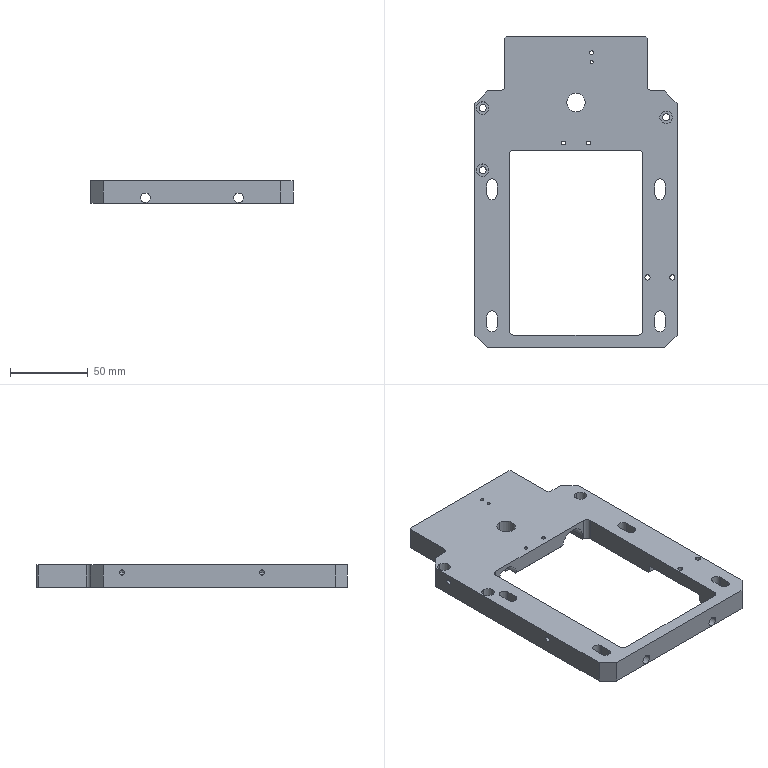NC program | NX | posted with a generic post | part box 130 x 200 x 14.5 mm
Whole program:
N10 G17 G21 G94 G90
(DRILLING_COPY_2 , TOOL : ZXZ)
N12 T21 M6
N14 G54
N16 G17 G0 G90 X15. Y-0.75 B0. C0. S3500 M3
N18 G43 Z30. H21
N20 G94 G81 G98 Z-1. F250. R3.
N22 X-15.
N24 X42.5
N26 X-42.5
N28 G80
N30 G0 X-42.5 Y-0.75 Z30.
N32 M5
(DRILLING_COPY_1_COPY_1 , TOOL : 3.3ZT)
N34 T13 M6
N36 G54
N38 G17 G0 G90 X15. Y-0.75 B0. C0. S2000 M3
N40 G43 Z30. H13
N42 G94 G83 G98 Z-15.091 F150. Q2. R3.
N44 X-15.
N46 G80
N48 G0 X-15. Y-0.75 Z30.
N50 M5
(DRILLING_COPY_COPY_COPY , TOOL : 2.5ZT)
N52 T22 M6
N54 G54
N56 G17 G0 G90 X-42.5 Y-0.75 B0. C0. S2000 M3
N58 G43 Z30. H22
N60 G94 G83 G98 Z-5. F150. Q2. R3.
N62 X42.5
N64 G80
N66 G0 X42.5 Y-0.75 Z30.
N68 M5
(HOLE_MILLING_2 , TOOL : D2)
N70 T18 M6
N72 G54
N74 G17 G0 G90 X-42.5 Y-0.75 B0. C0. S7500 M3
N76 G43 Z30. H18
N78 Z0.5
N80 G94 G3 X-42.735 Y-0.515 R0.235 F800.
N82 X-42.97 Y-0.75 R0.235
N84 X-42.97 Y-0.75 Z0.475 I0.47 J0.
N86 X-42.97 Y-0.75 Z0.45 I0.47 J0.
N88 X-42.97 Y-0.75 Z0.425 I0.47 J0.
N90 X-42.97 Y-0.75 Z0.4 I0.47 J0.
N92 X-42.97 Y-0.75 Z0.375 I0.47 J0.
N94 X-42.97 Y-0.75 Z0.35 I0.47 J0.
N96 X-42.97 Y-0.75 Z0.325 I0.47 J0.
N98 X-42.97 Y-0.75 Z0.3 I0.47 J0.
N100 X-42.97 Y-0.75 Z0.275 I0.47 J0.
N102 X-42.97 Y-0.75 Z0.25 I0.47 J0.
N104 X-42.97 Y-0.75 Z0.225 I0.47 J0.
N106 X-42.97 Y-0.75 Z0.2 I0.47 J0.
N108 X-42.97 Y-0.75 Z0.175 I0.47 J0.
N110 X-42.97 Y-0.75 Z0.15 I0.47 J0.
N112 X-42.97 Y-0.75 Z0.125 I0.47 J0.
N114 X-42.97 Y-0.75 Z0.1 I0.47 J0.
N116 X-42.97 Y-0.75 Z0.075 I0.47 J0.
N118 X-42.97 Y-0.75 Z0.05 I0.47 J0.
N120 X-42.97 Y-0.75 Z0.025 I0.47 J0.
N122 X-42.97 Y-0.75 Z0. I0.47 J0.
N124 X-42.97 Y-0.75 Z-0.025 I0.47 J0.
N126 X-42.97 Y-0.75 Z-0.05 I0.47 J0.
N128 X-42.97 Y-0.75 Z-0.075 I0.47 J0.
N130 X-42.97 Y-0.75 Z-0.1 I0.47 J0.
N132 X-42.97 Y-0.75 Z-0.125 I0.47 J0.
N134 X-42.97 Y-0.75 Z-0.15 I0.47 J0.
N136 X-42.97 Y-0.75 Z-0.175 I0.47 J0.
N138 X-42.97 Y-0.75 Z-0.2 I0.47 J0.
N140 X-42.97 Y-0.75 Z-0.225 I0.47 J0.
N142 X-42.97 Y-0.75 Z-0.25 I0.47 J0.
N144 X-42.97 Y-0.75 Z-0.275 I0.47 J0.
N146 X-42.97 Y-0.75 Z-0.3 I0.47 J0.
N148 X-42.97 Y-0.75 Z-0.325 I0.47 J0.
N150 X-42.97 Y-0.75 Z-0.35 I0.47 J0.
N152 X-42.97 Y-0.75 Z-0.375 I0.47 J0.
N154 X-42.97 Y-0.75 Z-0.4 I0.47 J0.
N156 X-42.97 Y-0.75 Z-0.425 I0.47 J0.
N158 X-42.97 Y-0.75 Z-0.45 I0.47 J0.
N160 X-42.97 Y-0.75 Z-0.475 I0.47 J0.
N162 X-42.97 Y-0.75 Z-0.5 I0.47 J0.
N164 X-42.97 Y-0.75 Z-0.525 I0.47 J0.
N166 X-42.97 Y-0.75 Z-0.55 I0.47 J0.
N168 X-42.97 Y-0.75 Z-0.575 I0.47 J0.
N170 X-42.97 Y-0.75 Z-0.6 I0.47 J0.
N172 X-42.97 Y-0.75 Z-0.625 I0.47 J0.
N174 X-42.97 Y-0.75 Z-0.65 I0.47 J0.
N176 X-42.97 Y-0.75 Z-0.675 I0.47 J0.
N178 X-42.97 Y-0.75 Z-0.7 I0.47 J0.
N180 X-42.97 Y-0.75 Z-0.725 I0.47 J0.
N182 X-42.97 Y-0.75 Z-0.75 I0.47 J0.
N184 X-42.97 Y-0.75 Z-0.775 I0.47 J0.
N186 X-42.97 Y-0.75 Z-0.8 I0.47 J0.
N188 X-42.97 Y-0.75 Z-0.825 I0.47 J0.
N190 X-42.97 Y-0.75 Z-0.85 I0.47 J0.
N192 X-42.97 Y-0.75 Z-0.875 I0.47 J0.
N194 X-42.97 Y-0.75 Z-0.9 I0.47 J0.
N196 X-42.97 Y-0.75 Z-0.925 I0.47 J0.
N198 X-42.97 Y-0.75 Z-0.95 I0.47 J0.
N200 X-42.97 Y-0.75 Z-0.975 I0.47 J0.
N202 X-42.97 Y-0.75 Z-1. I0.47 J0.
N204 X-42.97 Y-0.75 Z-1.025 I0.47 J0.
N206 X-42.97 Y-0.75 Z-1.05 I0.47 J0.
N208 X-42.97 Y-0.75 Z-1.075 I0.47 J0.
N210 X-42.97 Y-0.75 Z-1.1 I0.47 J0.
N212 X-42.97 Y-0.75 Z-1.125 I0.47 J0.
N214 X-42.97 Y-0.75 Z-1.15 I0.47 J0.
N216 X-42.97 Y-0.75 Z-1.175 I0.47 J0.
N218 X-42.97 Y-0.75 Z-1.2 I0.47 J0.
N220 X-42.97 Y-0.75 Z-1.225 I0.47 J0.
N222 X-42.97 Y-0.75 Z-1.25 I0.47 J0.
N224 X-42.97 Y-0.75 Z-1.275 I0.47 J0.
N226 X-42.97 Y-0.75 Z-1.3 I0.47 J0.
N228 X-42.97 Y-0.75 Z-1.325 I0.47 J0.
N230 X-42.97 Y-0.75 Z-1.35 I0.47 J0.
N232 X-42.97 Y-0.75 Z-1.375 I0.47 J0.
N234 X-42.97 Y-0.75 Z-1.4 I0.47 J0.
N236 X-42.97 Y-0.75 Z-1.425 I0.47 J0.
N238 X-42.97 Y-0.75 Z-1.45 I0.47 J0.
N240 X-42.97 Y-0.75 Z-1.475 I0.47 J0.
N242 X-42.97 Y-0.75 Z-1.5 I0.47 J0.
N244 X-42.97 Y-0.75 Z-1.525 I0.47 J0.
N246 X-42.97 Y-0.75 Z-1.55 I0.47 J0.
N248 X-42.97 Y-0.75 Z-1.575 I0.47 J0.
N250 X-42.97 Y-0.75 Z-1.6 I0.47 J0.
N252 X-42.97 Y-0.75 Z-1.625 I0.47 J0.
N254 X-42.97 Y-0.75 Z-1.65 I0.47 J0.
N256 X-42.97 Y-0.75 Z-1.675 I0.47 J0.
N258 X-42.97 Y-0.75 Z-1.7 I0.47 J0.
N260 X-42.97 Y-0.75 Z-1.725 I0.47 J0.
N262 X-42.97 Y-0.75 Z-1.75 I0.47 J0.
N264 X-42.97 Y-0.75 Z-1.775 I0.47 J0.
N266 X-42.97 Y-0.75 Z-1.8 I0.47 J0.
N268 X-42.97 Y-0.75 Z-1.825 I0.47 J0.
N270 X-42.97 Y-0.75 Z-1.85 I0.47 J0.
N272 X-42.97 Y-0.75 Z-1.875 I0.47 J0.
N274 X-42.97 Y-0.75 Z-1.9 I0.47 J0.
N276 X-42.97 Y-0.75 Z-1.925 I0.47 J0.
N278 X-42.97 Y-0.75 Z-1.95 I0.47 J0.
N280 X-42.97 Y-0.75 Z-1.975 I0.47 J0.
N282 X-42.97 Y-0.75 Z-2. I0.47 J0.
N284 X-42.97 Y-0.75 Z-2.025 I0.47 J0.
N286 X-42.97 Y-0.75 Z-2.05 I0.47 J0.
N288 X-42.97 Y-0.75 Z-2.075 I0.47 J0.
N290 X-42.97 Y-0.75 Z-2.1 I0.47 J0.
N292 X-42.97 Y-0.75 Z-2.125 I0.47 J0.
N294 X-42.97 Y-0.75 Z-2.15 I0.47 J0.
N296 X-42.97 Y-0.75 Z-2.175 I0.47 J0.
N298 X-42.97 Y-0.75 Z-2.2 I0.47 J0.
N300 X-42.97 Y-0.75 Z-2.225 I0.47 J0.
N302 X-42.97 Y-0.75 Z-2.25 I0.47 J0.
N304 X-42.97 Y-0.75 Z-2.275 I0.47 J0.
N306 X-42.97 Y-0.75 Z-2.3 I0.47 J0.
N308 X-42.97 Y-0.75 Z-2.325 I0.47 J0.
N310 X-42.97 Y-0.75 Z-2.35 I0.47 J0.
N312 X-42.97 Y-0.75 Z-2.375 I0.47 J0.
N314 X-42.97 Y-0.75 Z-2.4 I0.47 J0.
N316 X-42.97 Y-0.75 Z-2.425 I0.47 J0.
N318 X-42.97 Y-0.75 Z-2.45 I0.47 J0.
N320 X-42.97 Y-0.75 Z-2.475 I0.47 J0.
N322 X-42.97 Y-0.75 Z-2.5 I0.47 J0.
N324 X-42.97 Y-0.75 Z-2.525 I0.47 J0.
N326 X-42.97 Y-0.75 Z-2.55 I0.47 J0.
N328 X-42.97 Y-0.75 Z-2.575 I0.47 J0.
N330 X-42.97 Y-0.75 Z-2.6 I0.47 J0.
N332 X-42.97 Y-0.75 Z-2.625 I0.47 J0.
N334 X-42.97 Y-0.75 Z-2.65 I0.47 J0.
N336 X-42.97 Y-0.75 Z-2.675 I0.47 J0.
N338 X-42.97 Y-0.75 Z-2.7 I0.47 J0.
N340 X-42.97 Y-0.75 Z-2.725 I0.47 J0.
N342 X-42.97 Y-0.75 Z-2.75 I0.47 J0.
N344 X-42.97 Y-0.75 Z-2.775 I0.47 J0.
N346 X-42.97 Y-0.75 Z-2.8 I0.47 J0.
N348 X-42.97 Y-0.75 Z-2.825 I0.47 J0.
N350 X-42.97 Y-0.75 Z-2.85 I0.47 J0.
N352 X-42.97 Y-0.75 Z-2.875 I0.47 J0.
N354 X-42.97 Y-0.75 Z-2.9 I0.47 J0.
N356 X-42.97 Y-0.75 Z-2.925 I0.47 J0.
N358 X-42.97 Y-0.75 Z-2.95 I0.47 J0.
N360 X-42.97 Y-0.75 Z-2.975 I0.47 J0.
N362 X-42.97 Y-0.75 Z-3. I0.47 J0.
N364 X-42.97 Y-0.75 Z-3.025 I0.47 J0.
N366 X-42.97 Y-0.75 Z-3.05 I0.47 J0.
N368 X-42.97 Y-0.75 Z-3.075 I0.47 J0.
N370 X-42.97 Y-0.75 Z-3.1 I0.47 J0.
N372 X-42.97 Y-0.75 Z-3.125 I0.47 J0.
N374 X-42.97 Y-0.75 Z-3.15 I0.47 J0.
N376 X-42.97 Y-0.75 Z-3.175 I0.47 J0.
N378 X-42.97 Y-0.75 Z-3.2 I0.47 J0.
N380 X-42.97 Y-0.75 Z-3.225 I0.47 J0.
N382 X-42.97 Y-0.75 Z-3.25 I0.47 J0.
N384 X-42.97 Y-0.75 Z-3.275 I0.47 J0.
N386 X-42.97 Y-0.75 Z-3.3 I0.47 J0.
N388 X-42.97 Y-0.75 Z-3.325 I0.47 J0.
N390 X-42.97 Y-0.75 Z-3.35 I0.47 J0.
N392 X-42.97 Y-0.75 Z-3.375 I0.47 J0.
N394 X-42.97 Y-0.75 Z-3.4 I0.47 J0.
N396 X-42.97 Y-0.75 Z-3.425 I0.47 J0.
N398 X-42.97 Y-0.75 Z-3.45 I0.47 J0.
N400 X-42.97 Y-0.75 Z-3.475 I0.47 J0.
N402 X-42.97 Y-0.75 Z-3.5 I0.47 J0.
N404 X-42.97 Y-0.75 Z-3.525 I0.47 J0.
N406 X-42.97 Y-0.75 Z-3.55 I0.47 J0.
N408 X-42.97 Y-0.75 Z-3.575 I0.47 J0.
N410 X-42.97 Y-0.75 Z-3.6 I0.47 J0.
N412 X-42.97 Y-0.75 Z-3.625 I0.47 J0.
N414 X-42.97 Y-0.75 Z-3.65 I0.47 J0.
N416 X-42.97 Y-0.75 Z-3.675 I0.47 J0.
N418 X-42.97 Y-0.75 Z-3.7 I0.47 J0.
N420 X-42.97 Y-0.75 Z-3.725 I0.47 J0.
N422 X-42.97 Y-0.75 Z-3.75 I0.47 J0.
N424 X-42.97 Y-0.75 Z-3.775 I0.47 J0.
N426 X-42.97 Y-0.75 Z-3.8 I0.47 J0.
N428 X-42.97 Y-0.75 Z-3.825 I0.47 J0.
N430 X-42.97 Y-0.75 Z-3.85 I0.47 J0.
N432 X-42.97 Y-0.75 Z-3.875 I0.47 J0.
N434 X-42.97 Y-0.75 Z-3.9 I0.47 J0.
N436 X-42.97 Y-0.75 Z-3.925 I0.47 J0.
N438 X-42.97 Y-0.75 Z-3.95 I0.47 J0.
N440 X-42.97 Y-0.75 Z-3.975 I0.47 J0.
N442 X-42.97 Y-0.75 Z-4. I0.47 J0.
N444 X-42.97 Y-0.75 Z-4.025 I0.47 J0.
N446 X-42.97 Y-0.75 Z-4.05 I0.47 J0.
N448 X-42.97 Y-0.75 Z-4.075 I0.47 J0.
N450 X-42.97 Y-0.75 Z-4.1 I0.47 J0.
N452 X-42.97 Y-0.75 Z-4.125 I0.47 J0.
N454 X-42.97 Y-0.75 Z-4.15 I0.47 J0.
N456 X-42.97 Y-0.75 Z-4.175 I0.47 J0.
N458 X-42.97 Y-0.75 Z-4.2 I0.47 J0.
N460 X-42.97 Y-0.75 Z-4.225 I0.47 J0.
N462 X-42.97 Y-0.75 Z-4.25 I0.47 J0.
N464 X-42.97 Y-0.75 Z-4.275 I0.47 J0.
N466 X-42.97 Y-0.75 Z-4.3 I0.47 J0.
N468 X-42.97 Y-0.75 Z-4.325 I0.47 J0.
N470 X-42.97 Y-0.75 Z-4.35 I0.47 J0.
N472 X-42.97 Y-0.75 Z-4.375 I0.47 J0.
N474 X-42.97 Y-0.75 Z-4.4 I0.47 J0.
N476 X-42.97 Y-0.75 Z-4.425 I0.47 J0.
N478 X-42.97 Y-0.75 Z-4.45 I0.47 J0.
N480 X-42.97 Y-0.75 Z-4.475 I0.47 J0.
N482 X-42.97 Y-0.75 Z-4.5 I0.47 J0.
N484 X-42.97 Y-0.75 Z-4.525 I0.47 J0.
N486 X-42.97 Y-0.75 Z-4.55 I0.47 J0.
N488 X-42.97 Y-0.75 Z-4.575 I0.47 J0.
N490 X-42.97 Y-0.75 Z-4.6 I0.47 J0.
N492 X-42.97 Y-0.75 Z-4.625 I0.47 J0.
N494 X-42.97 Y-0.75 Z-4.65 I0.47 J0.
N496 X-42.97 Y-0.75 Z-4.675 I0.47 J0.
N498 X-42.97 Y-0.75 Z-4.7 I0.47 J0.
N500 X-42.97 Y-0.75 Z-4.725 I0.47 J0.
N502 X-42.97 Y-0.75 Z-4.75 I0.47 J0.
N504 X-42.97 Y-0.75 Z-4.775 I0.47 J0.
N506 X-42.97 Y-0.75 Z-4.8 I0.47 J0.
N508 X-42.97 Y-0.75 Z-4.825 I0.47 J0.
N510 X-42.97 Y-0.75 Z-4.85 I0.47 J0.
N512 X-42.97 Y-0.75 Z-4.875 I0.47 J0.
N514 X-42.97 Y-0.75 Z-4.9 I0.47 J0.
N516 X-42.97 Y-0.75 Z-4.925 I0.47 J0.
N518 X-42.97 Y-0.75 Z-4.95 I0.47 J0.
N520 X-42.97 Y-0.75 Z-4.975 I0.47 J0.
N522 X-42.97 Y-0.75 Z-5. I0.47 J0.
N524 X-42.5 Y-1.22 R0.47
N526 X-42.97 Y-0.75 R-0.47
N528 X-42.735 Y-0.985 R0.235
N530 X-42.5 Y-0.75 R0.235
N532 G0 Z30.
N534 X42.5
N536 Z0.5
N538 G3 X42.265 Y-0.515 R0.235
N540 X42.03 Y-0.75 R0.235
N542 X42.03 Y-0.75 Z0.475 I0.47 J0.
N544 X42.03 Y-0.75 Z0.45 I0.47 J0.
N546 X42.03 Y-0.75 Z0.425 I0.47 J0.
N548 X42.03 Y-0.75 Z0.4 I0.47 J0.
N550 X42.03 Y-0.75 Z0.375 I0.47 J0.
N552 X42.03 Y-0.75 Z0.35 I0.47 J0.
N554 X42.03 Y-0.75 Z0.325 I0.47 J0.
N556 X42.03 Y-0.75 Z0.3 I0.47 J0.
N558 X42.03 Y-0.75 Z0.275 I0.47 J0.
N560 X42.03 Y-0.75 Z0.25 I0.47 J0.
N562 X42.03 Y-0.75 Z0.225 I0.47 J0.
N564 X42.03 Y-0.75 Z0.2 I0.47 J0.
N566 X42.03 Y-0.75 Z0.175 I0.47 J0.
N568 X42.03 Y-0.75 Z0.15 I0.47 J0.
N570 X42.03 Y-0.75 Z0.125 I0.47 J0.
N572 X42.03 Y-0.75 Z0.1 I0.47 J0.
N574 X42.03 Y-0.75 Z0.075 I0.47 J0.
N576 X42.03 Y-0.75 Z0.05 I0.47 J0.
N578 X42.03 Y-0.75 Z0.025 I0.47 J0.
N580 X42.03 Y-0.75 Z0. I0.47 J0.
N582 X42.03 Y-0.75 Z-0.025 I0.47 J0.
N584 X42.03 Y-0.75 Z-0.05 I0.47 J0.
N586 X42.03 Y-0.75 Z-0.075 I0.47 J0.
N588 X42.03 Y-0.75 Z-0.1 I0.47 J0.
N590 X42.03 Y-0.75 Z-0.125 I0.47 J0.
N592 X42.03 Y-0.75 Z-0.15 I0.47 J0.
N594 X42.03 Y-0.75 Z-0.175 I0.47 J0.
N596 X42.03 Y-0.75 Z-0.2 I0.47 J0.
N598 X42.03 Y-0.75 Z-0.225 I0.47 J0.
N600 X42.03 Y-0.75 Z-0.25 I0.47 J0.
N602 X42.03 Y-0.75 Z-0.275 I0.47 J0.
N604 X42.03 Y-0.75 Z-0.3 I0.47 J0.
N606 X42.03 Y-0.75 Z-0.325 I0.47 J0.
N608 X42.03 Y-0.75 Z-0.35 I0.47 J0.
N610 X42.03 Y-0.75 Z-0.375 I0.47 J0.
N612 X42.03 Y-0.75 Z-0.4 I0.47 J0.
N614 X42.03 Y-0.75 Z-0.425 I0.47 J0.
N616 X42.03 Y-0.75 Z-0.45 I0.47 J0.
N618 X42.03 Y-0.75 Z-0.475 I0.47 J0.
N620 X42.03 Y-0.75 Z-0.5 I0.47 J0.
N622 X42.03 Y-0.75 Z-0.525 I0.47 J0.
N624 X42.03 Y-0.75 Z-0.55 I0.47 J0.
N626 X42.03 Y-0.75 Z-0.575 I0.47 J0.
N628 X42.03 Y-0.75 Z-0.6 I0.47 J0.
N630 X42.03 Y-0.75 Z-0.625 I0.47 J0.
N632 X42.03 Y-0.75 Z-0.65 I0.47 J0.
N634 X42.03 Y-0.75 Z-0.675 I0.47 J0.
N636 X42.03 Y-0.75 Z-0.7 I0.47 J0.
N638 X42.03 Y-0.75 Z-0.725 I0.47 J0.
N640 X42.03 Y-0.75 Z-0.75 I0.47 J0.
N642 X42.03 Y-0.75 Z-0.775 I0.47 J0.
N644 X42.03 Y-0.75 Z-0.8 I0.47 J0.
N646 X42.03 Y-0.75 Z-0.825 I0.47 J0.
N648 X42.03 Y-0.75 Z-0.85 I0.47 J0.
N650 X42.03 Y-0.75 Z-0.875 I0.47 J0.
N652 X42.03 Y-0.75 Z-0.9 I0.47 J0.
N654 X42.03 Y-0.75 Z-0.925 I0.47 J0.
N656 X42.03 Y-0.75 Z-0.95 I0.47 J0.
N658 X42.03 Y-0.75 Z-0.975 I0.47 J0.
N660 X42.03 Y-0.75 Z-1. I0.47 J0.
N662 X42.03 Y-0.75 Z-1.025 I0.47 J0.
N664 X42.03 Y-0.75 Z-1.05 I0.47 J0.
N666 X42.03 Y-0.75 Z-1.075 I0.47 J0.
N668 X42.03 Y-0.75 Z-1.1 I0.47 J0.
N670 X42.03 Y-0.75 Z-1.125 I0.47 J0.
N672 X42.03 Y-0.75 Z-1.15 I0.47 J0.
N674 X42.03 Y-0.75 Z-1.175 I0.47 J0.
N676 X42.03 Y-0.75 Z-1.2 I0.47 J0.
N678 X42.03 Y-0.75 Z-1.225 I0.47 J0.
N680 X42.03 Y-0.75 Z-1.25 I0.47 J0.
N682 X42.03 Y-0.75 Z-1.275 I0.47 J0.
N684 X42.03 Y-0.75 Z-1.3 I0.47 J0.
N686 X42.03 Y-0.75 Z-1.325 I0.47 J0.
N688 X42.03 Y-0.75 Z-1.35 I0.47 J0.
N690 X42.03 Y-0.75 Z-1.375 I0.47 J0.
N692 X42.03 Y-0.75 Z-1.4 I0.47 J0.
N694 X42.03 Y-0.75 Z-1.425 I0.47 J0.
N696 X42.03 Y-0.75 Z-1.45 I0.47 J0.
N698 X42.03 Y-0.75 Z-1.475 I0.47 J0.
N700 X42.03 Y-0.75 Z-1.5 I0.47 J0.
N702 X42.03 Y-0.75 Z-1.525 I0.47 J0.
N704 X42.03 Y-0.75 Z-1.55 I0.47 J0.
N706 X42.03 Y-0.75 Z-1.575 I0.47 J0.
N708 X42.03 Y-0.75 Z-1.6 I0.47 J0.
N710 X42.03 Y-0.75 Z-1.625 I0.47 J0.
N712 X42.03 Y-0.75 Z-1.65 I0.47 J0.
N714 X42.03 Y-0.75 Z-1.675 I0.47 J0.
N716 X42.03 Y-0.75 Z-1.7 I0.47 J0.
N718 X42.03 Y-0.75 Z-1.725 I0.47 J0.
N720 X42.03 Y-0.75 Z-1.75 I0.47 J0.
N722 X42.03 Y-0.75 Z-1.775 I0.47 J0.
N724 X42.03 Y-0.75 Z-1.8 I0.47 J0.
N726 X42.03 Y-0.75 Z-1.825 I0.47 J0.
N728 X42.03 Y-0.75 Z-1.85 I0.47 J0.
N730 X42.03 Y-0.75 Z-1.875 I0.47 J0.
N732 X42.03 Y-0.75 Z-1.9 I0.47 J0.
N734 X42.03 Y-0.75 Z-1.925 I0.47 J0.
N736 X42.03 Y-0.75 Z-1.95 I0.47 J0.
N738 X42.03 Y-0.75 Z-1.975 I0.47 J0.
N740 X42.03 Y-0.75 Z-2. I0.47 J0.
N742 X42.03 Y-0.75 Z-2.025 I0.47 J0.
N744 X42.03 Y-0.75 Z-2.05 I0.47 J0.
N746 X42.03 Y-0.75 Z-2.075 I0.47 J0.
N748 X42.03 Y-0.75 Z-2.1 I0.47 J0.
N750 X42.03 Y-0.75 Z-2.125 I0.47 J0.
N752 X42.03 Y-0.75 Z-2.15 I0.47 J0.
N754 X42.03 Y-0.75 Z-2.175 I0.47 J0.
N756 X42.03 Y-0.75 Z-2.2 I0.47 J0.
N758 X42.03 Y-0.75 Z-2.225 I0.47 J0.
N760 X42.03 Y-0.75 Z-2.25 I0.47 J0.
N762 X42.03 Y-0.75 Z-2.275 I0.47 J0.
N764 X42.03 Y-0.75 Z-2.3 I0.47 J0.
N766 X42.03 Y-0.75 Z-2.325 I0.47 J0.
N768 X42.03 Y-0.75 Z-2.35 I0.47 J0.
N770 X42.03 Y-0.75 Z-2.375 I0.47 J0.
N772 X42.03 Y-0.75 Z-2.4 I0.47 J0.
N774 X42.03 Y-0.75 Z-2.425 I0.47 J0.
N776 X42.03 Y-0.75 Z-2.45 I0.47 J0.
N778 X42.03 Y-0.75 Z-2.475 I0.47 J0.
N780 X42.03 Y-0.75 Z-2.5 I0.47 J0.
N782 X42.03 Y-0.75 Z-2.525 I0.47 J0.
N784 X42.03 Y-0.75 Z-2.55 I0.47 J0.
N786 X42.03 Y-0.75 Z-2.575 I0.47 J0.
N788 X42.03 Y-0.75 Z-2.6 I0.47 J0.
N790 X42.03 Y-0.75 Z-2.625 I0.47 J0.
N792 X42.03 Y-0.75 Z-2.65 I0.47 J0.
N794 X42.03 Y-0.75 Z-2.675 I0.47 J0.
N796 X42.03 Y-0.75 Z-2.7 I0.47 J0.
N798 X42.03 Y-0.75 Z-2.725 I0.47 J0.
N800 X42.03 Y-0.75 Z-2.75 I0.47 J0.
N802 X42.03 Y-0.75 Z-2.775 I0.47 J0.
N804 X42.03 Y-0.75 Z-2.8 I0.47 J0.
N806 X42.03 Y-0.75 Z-2.825 I0.47 J0.
N808 X42.03 Y-0.75 Z-2.85 I0.47 J0.
N810 X42.03 Y-0.75 Z-2.875 I0.47 J0.
N812 X42.03 Y-0.75 Z-2.9 I0.47 J0.
N814 X42.03 Y-0.75 Z-2.925 I0.47 J0.
N816 X42.03 Y-0.75 Z-2.95 I0.47 J0.
N818 X42.03 Y-0.75 Z-2.975 I0.47 J0.
N820 X42.03 Y-0.75 Z-3. I0.47 J0.
N822 X42.03 Y-0.75 Z-3.025 I0.47 J0.
N824 X42.03 Y-0.75 Z-3.05 I0.47 J0.
N826 X42.03 Y-0.75 Z-3.075 I0.47 J0.
N828 X42.03 Y-0.75 Z-3.1 I0.47 J0.
N830 X42.03 Y-0.75 Z-3.125 I0.47 J0.
N832 X42.03 Y-0.75 Z-3.15 I0.47 J0.
N834 X42.03 Y-0.75 Z-3.175 I0.47 J0.
N836 X42.03 Y-0.75 Z-3.2 I0.47 J0.
N838 X42.03 Y-0.75 Z-3.225 I0.47 J0.
N840 X42.03 Y-0.75 Z-3.25 I0.47 J0.
N842 X42.03 Y-0.75 Z-3.275 I0.47 J0.
N844 X42.03 Y-0.75 Z-3.3 I0.47 J0.
N846 X42.03 Y-0.75 Z-3.325 I0.47 J0.
N848 X42.03 Y-0.75 Z-3.35 I0.47 J0.
N850 X42.03 Y-0.75 Z-3.375 I0.47 J0.
N852 X42.03 Y-0.75 Z-3.4 I0.47 J0.
N854 X42.03 Y-0.75 Z-3.425 I0.47 J0.
N856 X42.03 Y-0.75 Z-3.45 I0.47 J0.
N858 X42.03 Y-0.75 Z-3.475 I0.47 J0.
N860 X42.03 Y-0.75 Z-3.5 I0.47 J0.
N862 X42.03 Y-0.75 Z-3.525 I0.47 J0.
N864 X42.03 Y-0.75 Z-3.55 I0.47 J0.
N866 X42.03 Y-0.75 Z-3.575 I0.47 J0.
N868 X42.03 Y-0.75 Z-3.6 I0.47 J0.
N870 X42.03 Y-0.75 Z-3.625 I0.47 J0.
N872 X42.03 Y-0.75 Z-3.65 I0.47 J0.
N874 X42.03 Y-0.75 Z-3.675 I0.47 J0.
N876 X42.03 Y-0.75 Z-3.7 I0.47 J0.
N878 X42.03 Y-0.75 Z-3.725 I0.47 J0.
N880 X42.03 Y-0.75 Z-3.75 I0.47 J0.
N882 X42.03 Y-0.75 Z-3.775 I0.47 J0.
N884 X42.03 Y-0.75 Z-3.8 I0.47 J0.
N886 X42.03 Y-0.75 Z-3.825 I0.47 J0.
N888 X42.03 Y-0.75 Z-3.85 I0.47 J0.
N890 X42.03 Y-0.75 Z-3.875 I0.47 J0.
N892 X42.03 Y-0.75 Z-3.9 I0.47 J0.
N894 X42.03 Y-0.75 Z-3.925 I0.47 J0.
N896 X42.03 Y-0.75 Z-3.95 I0.47 J0.
N898 X42.03 Y-0.75 Z-3.975 I0.47 J0.
N900 X42.03 Y-0.75 Z-4. I0.47 J0.
N902 X42.03 Y-0.75 Z-4.025 I0.47 J0.
N904 X42.03 Y-0.75 Z-4.05 I0.47 J0.
N906 X42.03 Y-0.75 Z-4.075 I0.47 J0.
N908 X42.03 Y-0.75 Z-4.1 I0.47 J0.
N910 X42.03 Y-0.75 Z-4.125 I0.47 J0.
N912 X42.03 Y-0.75 Z-4.15 I0.47 J0.
N914 X42.03 Y-0.75 Z-4.175 I0.47 J0.
N916 X42.03 Y-0.75 Z-4.2 I0.47 J0.
N918 X42.03 Y-0.75 Z-4.225 I0.47 J0.
N920 X42.03 Y-0.75 Z-4.25 I0.47 J0.
N922 X42.03 Y-0.75 Z-4.275 I0.47 J0.
N924 X42.03 Y-0.75 Z-4.3 I0.47 J0.
N926 X42.03 Y-0.75 Z-4.325 I0.47 J0.
N928 X42.03 Y-0.75 Z-4.35 I0.47 J0.
N930 X42.03 Y-0.75 Z-4.375 I0.47 J0.
N932 X42.03 Y-0.75 Z-4.4 I0.47 J0.
N934 X42.03 Y-0.75 Z-4.425 I0.47 J0.
N936 X42.03 Y-0.75 Z-4.45 I0.47 J0.
N938 X42.03 Y-0.75 Z-4.475 I0.47 J0.
N940 X42.03 Y-0.75 Z-4.5 I0.47 J0.
N942 X42.03 Y-0.75 Z-4.525 I0.47 J0.
N944 X42.03 Y-0.75 Z-4.55 I0.47 J0.
N946 X42.03 Y-0.75 Z-4.575 I0.47 J0.
N948 X42.03 Y-0.75 Z-4.6 I0.47 J0.
N950 X42.03 Y-0.75 Z-4.625 I0.47 J0.
N952 X42.03 Y-0.75 Z-4.65 I0.47 J0.
N954 X42.03 Y-0.75 Z-4.675 I0.47 J0.
N956 X42.03 Y-0.75 Z-4.7 I0.47 J0.
N958 X42.03 Y-0.75 Z-4.725 I0.47 J0.
N960 X42.03 Y-0.75 Z-4.75 I0.47 J0.
N962 X42.03 Y-0.75 Z-4.775 I0.47 J0.
N964 X42.03 Y-0.75 Z-4.8 I0.47 J0.
N966 X42.03 Y-0.75 Z-4.825 I0.47 J0.
N968 X42.03 Y-0.75 Z-4.85 I0.47 J0.
N970 X42.03 Y-0.75 Z-4.875 I0.47 J0.
N972 X42.03 Y-0.75 Z-4.9 I0.47 J0.
N974 X42.03 Y-0.75 Z-4.925 I0.47 J0.
N976 X42.03 Y-0.75 Z-4.95 I0.47 J0.
N978 X42.03 Y-0.75 Z-4.975 I0.47 J0.
N980 X42.03 Y-0.75 Z-5. I0.47 J0.
N982 X42.5 Y-1.22 R0.47
N984 X42.03 Y-0.75 R-0.47
N986 X42.265 Y-0.985 R0.235
N988 X42.5 Y-0.75 R0.235
N990 G0 Z30.
N992 M5
(DRILLING_COPY_2_COPY , TOOL : D6A45)
N994 T01 M6
N996 G54
N998 G17 G0 G90 X15. Y-0.75 B0. C0. S3500 M3
N1000 G43 Z30. H1
N1002 G94 G81 G98 Z-1.6 F250. R3.
N1004 X-15.
N1006 X42.5
N1008 X-42.5
N1010 G80
N1012 G0 X-42.5 Y-0.75 Z30.
N1014 M5
(刀补18 , TOOL : D2)
N1016 T18 M6
N1018 G54
N1020 G17 G0 G90 X-42.5 Y-0.75 B0. C0. S7500 M3
N1022 G43 Z30. H18
N1024 Z0.5
N1026 G41 G94 G1 X-42.524 Y-0.653 F800. D18
N1028 G3 X-42.98 Y-0.75 R0.238
N1030 X-42.98 Y-0.75 Z-0.5 I0.48 J0.
N1032 X-42.98 Y-0.75 Z-1.5 I0.48 J0.
N1034 X-42.98 Y-0.75 Z-2.5 I0.48 J0.
N1036 X-42.98 Y-0.75 Z-3.5 I0.48 J0.
N1038 X-42.98 Y-0.75 Z-4.5 I0.48 J0.
N1040 X-42.02 Y-0.75 Z-5. I0.48 J0.
N1042 X-42.5 Y-0.27 R0.48
N1044 X-42.02 Y-0.75 R-0.48
N1046 X-42.476 Y-0.653 R0.238
N1048 G40
N1050 G1 X-42.5 Y-0.75
N1052 G0 Z30.
N1054 X42.5
N1056 Z0.5
N1058 G41 G1 X42.476 Y-0.653
N1060 G3 X42.02 Y-0.75 R0.238
N1062 X42.02 Y-0.75 Z-0.5 I0.48 J0.
N1064 X42.02 Y-0.75 Z-1.5 I0.48 J0.
N1066 X42.02 Y-0.75 Z-2.5 I0.48 J0.
N1068 X42.02 Y-0.75 Z-3.5 I0.48 J0.
N1070 X42.02 Y-0.75 Z-4.5 I0.48 J0.
N1072 X42.98 Y-0.75 Z-5. I0.48 J0.
N1074 X42.5 Y-0.27 R0.48
N1076 X42.98 Y-0.75 R-0.48
N1078 X42.524 Y-0.653 R0.238
N1080 G40
N1082 G1 X42.5 Y-0.75
N1084 G0 Z30.
N1086 M5
N1088 M2